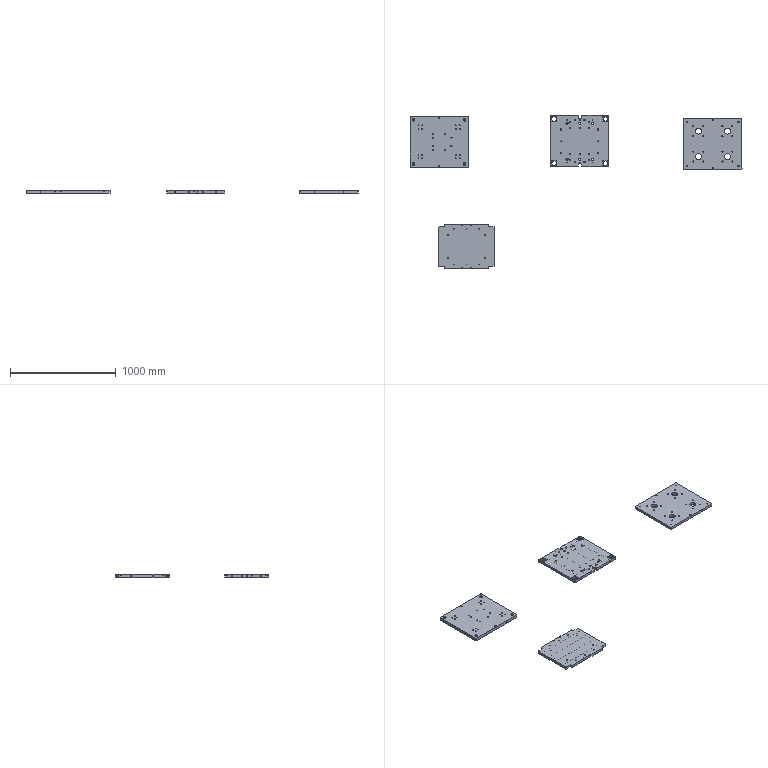NC program | Mastercam | posted with a generic post | part box 3140 x 1452 x 30 mm
Lines 1 to 480 of 5015:
%
O0000()
(MATERIAL - ALUMINUM MM - 2024)
( T16 | 16 FEM | H16 | XY STOCK TO LEAVE - .1 | Z STOCK TO LEAVE - .05 )
( T10 | 10 FEM | H10 | XY STOCK TO LEAVE - 0. | Z STOCK TO LEAVE - .05 )
( T7 | 4 CHM | H7 )
( T18 | 8.5 DR | H18 | XY STOCK TO LEAVE - 0. | Z STOCK TO LEAVE - .05 )
( T13 | 10 DR | H13 )
( T6 | 6 FEM | H6 | XY STOCK TO LEAVE - .05 | Z STOCK TO LEAVE - .05 )
N100 G21
N110 G0 G17 G40 G49 G80 G90
( ? )
N120 T16 M6
N130 G0 G90 G54 X-273.1 Y-220. A0. S6000 M3
N140 G43 H16 Z50. M8
N150 Z1.
N160 G1 Z-.499 F600.
N170 Y-180. F4000.
N180 Y180.
N190 Y220.
N200 Z-.998 F600.
N210 Y180. F4000.
N220 Y-180.
N230 Y-220.
N240 Z-1.497 F600.
N250 Y-180. F4000.
N260 Y180.
N270 Y220.
N280 Z-1.996 F600.
N290 Y180. F4000.
N300 Y-180.
N310 Y-220.
N320 Z-2.495 F600.
N330 Y-180. F4000.
N340 Y180.
N350 Y220.
N360 Z-2.994 F600.
N370 Y180. F4000.
N380 Y-180.
N390 Y-220.
N400 Z-3.493 F600.
N410 Y-180. F4000.
N420 Y180.
N430 Y220.
N440 Z-3.992 F600.
N450 Y180. F4000.
N460 Y-180.
N470 Y-220.
N480 Z-4.491 F600.
N490 Y-180. F4000.
N500 Y180.
N510 Y220.
N520 Z-4.99 F600.
N530 Y180. F4000.
N540 Y-180.
N550 Y-220.
N560 Z-5.489 F600.
N570 Y-180. F4000.
N580 Y180.
N590 Y220.
N600 Z-5.988 F600.
N610 Y180. F4000.
N620 Y-180.
N630 Y-220.
N640 Z-6.487 F600.
N650 Y-180. F4000.
N660 Y180.
N670 Y220.
N680 Z-6.986 F600.
N690 Y180. F4000.
N700 Y-180.
N710 Y-220.
N720 Z-7.485 F600.
N730 Y-180. F4000.
N740 Y180.
N750 Y220.
N760 Z-7.984 F600.
N770 Y180. F4000.
N780 Y-180.
N790 Y-220.
N800 Z-8.483 F600.
N810 Y-180. F4000.
N820 Y180.
N830 Y220.
N840 Z-8.982 F600.
N850 Y180. F4000.
N860 Y-180.
N870 Y-220.
N880 Z-9.481 F600.
N890 Y-180. F4000.
N900 Y180.
N910 Y220.
N920 Z-9.98 F600.
N930 Y180. F4000.
N940 Y-180.
N950 Y-220.
N960 Z-10.479 F600.
N970 Y-180. F4000.
N980 Y180.
N990 Y220.
N1000 Z-10.978 F600.
N1010 Y180. F4000.
N1020 Y-180.
N1030 Y-220.
N1040 Z-11.477 F600.
N1050 Y-180. F4000.
N1060 Y180.
N1070 Y220.
N1080 Z-11.976 F600.
N1090 Y180. F4000.
N1100 Y-180.
N1110 Y-220.
N1120 Z-12.475 F600.
N1130 Y-180. F4000.
N1140 Y180.
N1150 Y220.
N1160 Z-12.974 F600.
N1170 Y180. F4000.
N1180 Y-180.
N1190 Y-220.
N1200 Z-13.473 F600.
N1210 Y-180. F4000.
N1220 Y180.
N1230 Y220.
N1240 Z-13.972 F600.
N1250 Y180. F4000.
N1260 Y-180.
N1270 Y-220.
N1280 Z-14.471 F600.
N1290 Y-180. F4000.
N1300 Y180.
N1310 Y220.
N1320 Z-14.97 F600.
N1330 Y180. F4000.
N1340 Y-180.
N1350 Y-220.
N1360 Z-15.469 F600.
N1370 Y-180. F4000.
N1380 Y180.
N1390 Y220.
N1400 Z-15.968 F600.
N1410 Y180. F4000.
N1420 Y-180.
N1430 Y-220.
N1440 Z-16.467 F600.
N1450 Y-180. F4000.
N1460 Y180.
N1470 Y220.
N1480 Z-16.966 F600.
N1490 Y180. F4000.
N1500 Y-180.
N1510 Y-220.
N1520 Z-17.465 F600.
N1530 Y-180. F4000.
N1540 Y180.
N1550 Y220.
N1560 Z-17.964 F600.
N1570 Y180. F4000.
N1580 Y-180.
N1590 Y-220.
N1600 Z-18.463 F600.
N1610 Y-180. F4000.
N1620 Y180.
N1630 Y220.
N1640 Z-18.962 F600.
N1650 Y180. F4000.
N1660 Y-180.
N1670 Y-220.
N1680 Z-19.461 F600.
N1690 Y-180. F4000.
N1700 Y180.
N1710 Y220.
N1720 Z-19.96 F600.
N1730 Y180. F4000.
N1740 Y-180.
N1750 Y-220.
N1760 Z-20.459 F600.
N1770 Y-180. F4000.
N1780 Y180.
N1790 Y220.
N1800 Z-20.958 F600.
N1810 Y180. F4000.
N1820 Y-180.
N1830 Y-220.
N1840 Z-21.457 F600.
N1850 Y-180. F4000.
N1860 Y180.
N1870 Y220.
N1880 Z-21.956 F600.
N1890 Y180. F4000.
N1900 Y-180.
N1910 Y-220.
N1920 Z-22.455 F600.
N1930 Y-180. F4000.
N1940 Y180.
N1950 Y220.
N1960 Z-22.954 F600.
N1970 Y180. F4000.
N1980 Y-180.
N1990 Y-220.
N2000 Z-23.453 F600.
N2010 Y-180. F4000.
N2020 Y180.
N2030 Y220.
N2040 Z-23.952 F600.
N2050 Y180. F4000.
N2060 Y-180.
N2070 Y-220.
N2080 Z-24.451 F600.
N2090 Y-180. F4000.
N2100 Y180.
N2110 Y220.
N2120 Z-24.95 F600.
N2130 Y180. F4000.
N2140 Y-180.
N2150 Y-220.
N2160 G0 Z50.
N2170 X273.1 Y220.
N2180 Z1.
N2190 G1 Z-.499 F600.
N2200 Y180. F4000.
N2210 Y-180.
N2220 Y-220.
N2230 Z-.998 F600.
N2240 Y-180. F4000.
N2250 Y180.
N2260 Y220.
N2270 Z-1.497 F600.
N2280 Y180. F4000.
N2290 Y-180.
N2300 Y-220.
N2310 Z-1.996 F600.
N2320 Y-180. F4000.
N2330 Y180.
N2340 Y220.
N2350 Z-2.495 F600.
N2360 Y180. F4000.
N2370 Y-180.
N2380 Y-220.
N2390 Z-2.994 F600.
N2400 Y-180. F4000.
N2410 Y180.
N2420 Y220.
N2430 Z-3.493 F600.
N2440 Y180. F4000.
N2450 Y-180.
N2460 Y-220.
N2470 Z-3.992 F600.
N2480 Y-180. F4000.
N2490 Y180.
N2500 Y220.
N2510 Z-4.491 F600.
N2520 Y180. F4000.
N2530 Y-180.
N2540 Y-220.
N2550 Z-4.99 F600.
N2560 Y-180. F4000.
N2570 Y180.
N2580 Y220.
N2590 Z-5.489 F600.
N2600 Y180. F4000.
N2610 Y-180.
N2620 Y-220.
N2630 Z-5.988 F600.
N2640 Y-180. F4000.
N2650 Y180.
N2660 Y220.
N2670 Z-6.487 F600.
N2680 Y180. F4000.
N2690 Y-180.
N2700 Y-220.
N2710 Z-6.986 F600.
N2720 Y-180. F4000.
N2730 Y180.
N2740 Y220.
N2750 Z-7.485 F600.
N2760 Y180. F4000.
N2770 Y-180.
N2780 Y-220.
N2790 Z-7.984 F600.
N2800 Y-180. F4000.
N2810 Y180.
N2820 Y220.
N2830 Z-8.483 F600.
N2840 Y180. F4000.
N2850 Y-180.
N2860 Y-220.
N2870 Z-8.982 F600.
N2880 Y-180. F4000.
N2890 Y180.
N2900 Y220.
N2910 Z-9.481 F600.
N2920 Y180. F4000.
N2930 Y-180.
N2940 Y-220.
N2950 Z-9.98 F600.
N2960 Y-180. F4000.
N2970 Y180.
N2980 Y220.
N2990 Z-10.479 F600.
N3000 Y180. F4000.
N3010 Y-180.
N3020 Y-220.
N3030 Z-10.978 F600.
N3040 Y-180. F4000.
N3050 Y180.
N3060 Y220.
N3070 Z-11.477 F600.
N3080 Y180. F4000.
N3090 Y-180.
N3100 Y-220.
N3110 Z-11.976 F600.
N3120 Y-180. F4000.
N3130 Y180.
N3140 Y220.
N3150 Z-12.475 F600.
N3160 Y180. F4000.
N3170 Y-180.
N3180 Y-220.
N3190 Z-12.974 F600.
N3200 Y-180. F4000.
N3210 Y180.
N3220 Y220.
N3230 Z-13.473 F600.
N3240 Y180. F4000.
N3250 Y-180.
N3260 Y-220.
N3270 Z-13.972 F600.
N3280 Y-180. F4000.
N3290 Y180.
N3300 Y220.
N3310 Z-14.471 F600.
N3320 Y180. F4000.
N3330 Y-180.
N3340 Y-220.
N3350 Z-14.97 F600.
N3360 Y-180. F4000.
N3370 Y180.
N3380 Y220.
N3390 Z-15.469 F600.
N3400 Y180. F4000.
N3410 Y-180.
N3420 Y-220.
N3430 Z-15.968 F600.
N3440 Y-180. F4000.
N3450 Y180.
N3460 Y220.
N3470 Z-16.467 F600.
N3480 Y180. F4000.
N3490 Y-180.
N3500 Y-220.
N3510 Z-16.966 F600.
N3520 Y-180. F4000.
N3530 Y180.
N3540 Y220.
N3550 Z-17.465 F600.
N3560 Y180. F4000.
N3570 Y-180.
N3580 Y-220.
N3590 Z-17.964 F600.
N3600 Y-180. F4000.
N3610 Y180.
N3620 Y220.
N3630 Z-18.463 F600.
N3640 Y180. F4000.
N3650 Y-180.
N3660 Y-220.
N3670 Z-18.962 F600.
N3680 Y-180. F4000.
N3690 Y180.
N3700 Y220.
N3710 Z-19.461 F600.
N3720 Y180. F4000.
N3730 Y-180.
N3740 Y-220.
N3750 Z-19.96 F600.
N3760 Y-180. F4000.
N3770 Y180.
N3780 Y220.
N3790 Z-20.459 F600.
N3800 Y180. F4000.
N3810 Y-180.
N3820 Y-220.
N3830 Z-20.958 F600.
N3840 Y-180. F4000.
N3850 Y180.
N3860 Y220.
N3870 Z-21.457 F600.
N3880 Y180. F4000.
N3890 Y-180.
N3900 Y-220.
N3910 Z-21.956 F600.
N3920 Y-180. F4000.
N3930 Y180.
N3940 Y220.
N3950 Z-22.455 F600.
N3960 Y180. F4000.
N3970 Y-180.
N3980 Y-220.
N3990 Z-22.954 F600.
N4000 Y-180. F4000.
N4010 Y180.
N4020 Y220.
N4030 Z-23.453 F600.
N4040 Y180. F4000.
N4050 Y-180.
N4060 Y-220.
N4070 Z-23.952 F600.
N4080 Y-180. F4000.
N4090 Y180.
N4100 Y220.
N4110 Z-24.451 F600.
N4120 Y180. F4000.
N4130 Y-180.
N4140 Y-220.
N4150 Z-24.95 F600.
N4160 Y-180. F4000.
N4170 Y180.
N4180 Y220.
N4190 G0 Z50.
N4200 M5
N4210 G91 G28 Z0. M9
N4220 A0.
N4230 M01
N4240 T10 M6
N4250 G0 G90 G17 G54 X-270. Y-215. A0. S6000 M3
N4260 G43 H10 Z50. M8
N4270 Z1.
N4280 G1 Z-12.475 F600.
N4290 Y-180. F1000.
N4300 Y180.
N4310 Y215.
N4320 G0 Z50.
N4330 Y-215.
N4340 Z-11.475
N4350 G1 Z-24.95 F600.
N4360 Y-180. F1000.
N4370 Y180.
N4380 Y215.
N4390 G0 Z50.
N4400 X270.
N4410 Z1.
N4420 G1 Z-12.475 F600.
N4430 Y180. F1000.
N4440 Y-180.
N4450 Y-215.
N4460 G0 Z50.
N4470 Y215.
N4480 Z-11.475
N4490 G1 Z-24.95 F600.
N4500 Y180. F1000.
N4510 Y-180.
N4520 Y-215.
N4530 G0 Z50.
N4540 M5
N4550 G91 G28 Z0. M9
N4560 A0.
N4570 M01
N4580 T7 M6
N4590 G0 G90 G17 G54 X-265.65 Y-210. A0. S6000 M3
N4600 G43 H7 Z50. M8
N4610 Z1.
N4620 G1 Z-.75 F600.
N4630 Y-180. F1000.
N4640 Y180.
N4650 Y210.
N4660 G0 Z50.
N4670 X265.65
N4680 Z1.
N4690 G1 Z-.75 F600.
N4700 Y180. F1000.
N4710 Y-180.
N4720 Y-210.
N4730 G0 Z50.
N4740 M5
N4750 G91 G28 Z0. M9
N4760 A0.
N4770 M01
( ?X )
M00